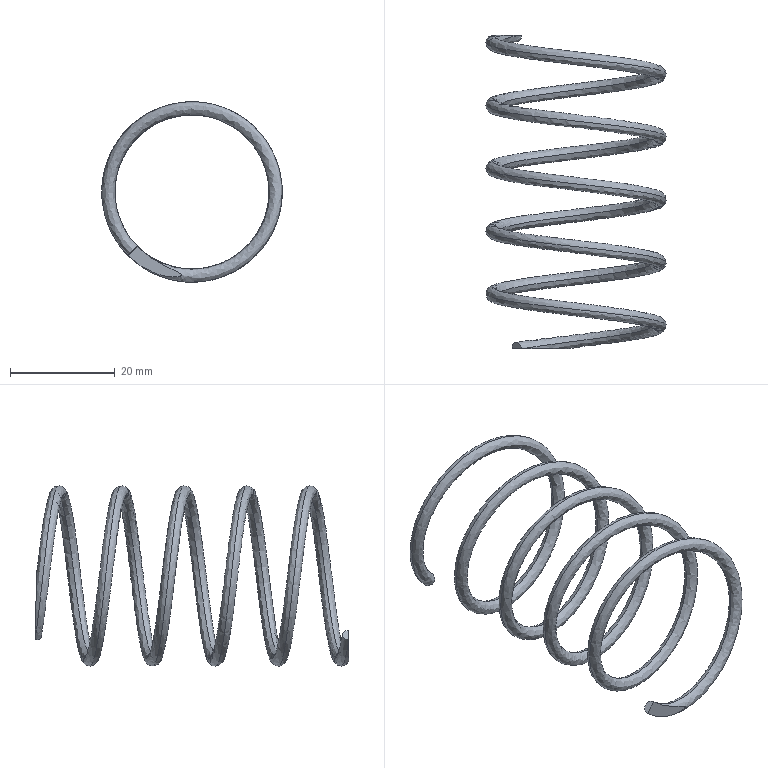Part | SolidWorks | features Helix 1, ICE 1, Sweep 1 | 1 solid | 7 faces | box 34.5 x 60 x 34.5 mm | volume 2448 mm3 | plane 5 | spline 2